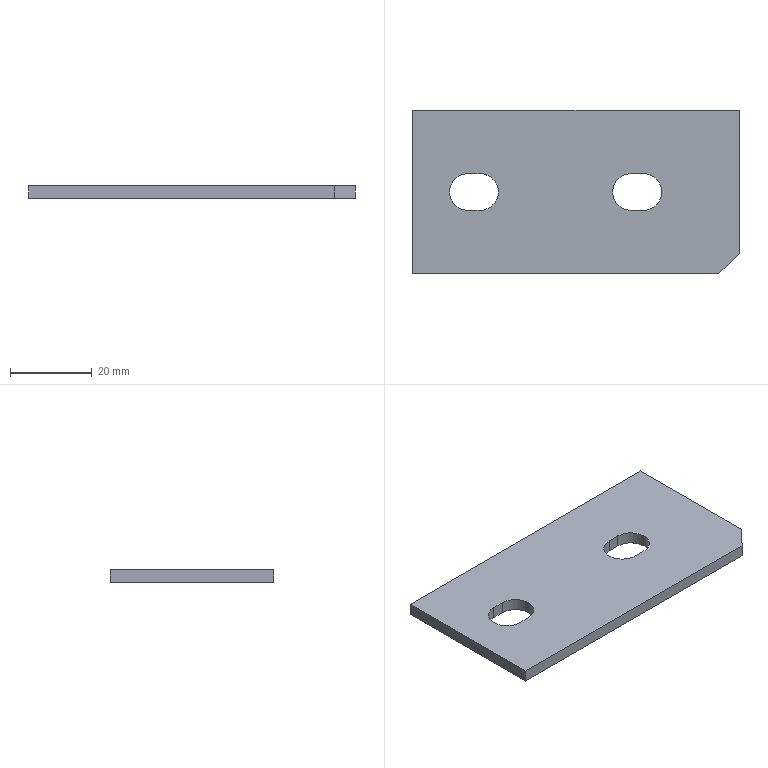Part | SolidWorks | features BaseBody 1 | 1 solid | 17 faces | box 80 x 40 x 3 mm | volume 9019 mm3 | plane 11 | cylinder 6 | commonest cylinder face diameters 9 x6
STEP:
#1=CARTESIAN_POINT('',(-26.5,-4.5,-3.));
#2=VERTEX_POINT('',#1);
#3=CARTESIAN_POINT('',(-26.5,-4.5,0.));
#4=VERTEX_POINT('',#3);
#5=CARTESIAN_POINT('',(-26.5,-4.5,-10.));
#6=DIRECTION('',(0.,0.,1.));
#7=VECTOR('',#6,1000.);
#8=LINE('',#5,#7);
#9=EDGE_CURVE('',#2,#4,#8,.T.);
#10=ORIENTED_EDGE('',*,*,#9,.T.);
#11=CARTESIAN_POINT('',(-23.5,-4.5,0.));
#12=VERTEX_POINT('',#11);
#13=CARTESIAN_POINT('',(-26.5,-4.5,0.));
#14=DIRECTION('',(1.,0.,0.));
#15=VECTOR('',#14,1000.);
#16=LINE('',#13,#15);
#17=EDGE_CURVE('',#4,#12,#16,.T.);
#18=ORIENTED_EDGE('',*,*,#17,.T.);
#19=CARTESIAN_POINT('',(-23.5,-4.5,-3.));
#20=VERTEX_POINT('',#19);
#21=CARTESIAN_POINT('',(-23.5,-4.5,-10.));
#22=DIRECTION('',(0.,0.,1.));
#23=VECTOR('',#22,1000.);
#24=LINE('',#21,#23);
#25=EDGE_CURVE('',#20,#12,#24,.T.);
#26=ORIENTED_EDGE('',*,*,#25,.F.);
#27=CARTESIAN_POINT('',(0.,-4.5,-3.));
#28=DIRECTION('',(1.,0.,0.));
#29=VECTOR('',#28,1000.);
#30=LINE('',#27,#29);
#31=EDGE_CURVE('',#2,#20,#30,.T.);
#32=ORIENTED_EDGE('',*,*,#31,.F.);
#33=EDGE_LOOP('',(#10,#18,#26,#32));
#34=FACE_OUTER_BOUND('',#33,.T.);
#35=CARTESIAN_POINT('',(-26.5,-4.5,-10.));
#36=DIRECTION('',(0.,-1.,0.));
#37=DIRECTION('',(0.,0.,-1.));
#38=AXIS2_PLACEMENT_3D('',#35,#36,#37);
#39=PLANE('',#38);
#40=ADVANCED_FACE('',(#34),#39,.F.);
#41=CARTESIAN_POINT('',(-19.,0.,-3.));
#42=VERTEX_POINT('',#41);
#43=CARTESIAN_POINT('',(-19.,0.,0.));
#44=VERTEX_POINT('',#43);
#45=CARTESIAN_POINT('',(-19.,0.,-10.));
#46=DIRECTION('',(0.,0.,1.));
#47=VECTOR('',#46,1000.);
#48=LINE('',#45,#47);
#49=EDGE_CURVE('',#42,#44,#48,.T.);
#50=ORIENTED_EDGE('',*,*,#49,.F.);
#51=CARTESIAN_POINT('',(-23.5,0.,-3.));
#52=DIRECTION('',(0.,0.,1.));
#53=DIRECTION('',(1.,0.,0.));
#54=AXIS2_PLACEMENT_3D('',#51,#52,#53);
#55=CIRCLE('',#54,4.5);
#56=EDGE_CURVE('',#20,#42,#55,.T.);
#57=ORIENTED_EDGE('',*,*,#56,.F.);
#58=ORIENTED_EDGE('',*,*,#25,.T.);
#59=CARTESIAN_POINT('',(-23.5,0.,0.));
#60=DIRECTION('',(0.,0.,1.));
#61=DIRECTION('',(1.,0.,0.));
#62=AXIS2_PLACEMENT_3D('',#59,#60,#61);
#63=CIRCLE('',#62,4.5);
#64=EDGE_CURVE('',#12,#44,#63,.T.);
#65=ORIENTED_EDGE('',*,*,#64,.T.);
#66=EDGE_LOOP('',(#50,#57,#58,#65));
#67=FACE_OUTER_BOUND('',#66,.T.);
#68=CARTESIAN_POINT('',(-23.5,0.,-10.));
#69=DIRECTION('',(0.,0.,1.));
#70=DIRECTION('',(1.,0.,0.));
#71=AXIS2_PLACEMENT_3D('',#68,#69,#70);
#72=CYLINDRICAL_SURFACE('',#71,4.5);
#73=ADVANCED_FACE('',(#67),#72,.F.);
#74=CARTESIAN_POINT('',(-23.5,4.5,-3.));
#75=VERTEX_POINT('',#74);
#76=CARTESIAN_POINT('',(-23.5,4.5,0.));
#77=VERTEX_POINT('',#76);
#78=CARTESIAN_POINT('',(-23.5,4.5,-10.));
#79=DIRECTION('',(0.,0.,1.));
#80=VECTOR('',#79,1000.);
#81=LINE('',#78,#80);
#82=EDGE_CURVE('',#75,#77,#81,.T.);
#83=ORIENTED_EDGE('',*,*,#82,.T.);
#84=CARTESIAN_POINT('',(-26.5,4.5,0.));
#85=VERTEX_POINT('',#84);
#86=CARTESIAN_POINT('',(-26.5,4.5,0.));
#87=DIRECTION('',(-1.,0.,0.));
#88=VECTOR('',#87,1000.);
#89=LINE('',#86,#88);
#90=EDGE_CURVE('',#77,#85,#89,.T.);
#91=ORIENTED_EDGE('',*,*,#90,.T.);
#92=CARTESIAN_POINT('',(-26.5,4.5,-3.));
#93=VERTEX_POINT('',#92);
#94=CARTESIAN_POINT('',(-26.5,4.5,-10.));
#95=DIRECTION('',(0.,0.,1.));
#96=VECTOR('',#95,1000.);
#97=LINE('',#94,#96);
#98=EDGE_CURVE('',#93,#85,#97,.T.);
#99=ORIENTED_EDGE('',*,*,#98,.F.);
#100=CARTESIAN_POINT('',(0.,4.5,-3.));
#101=DIRECTION('',(-1.,0.,0.));
#102=VECTOR('',#101,1000.);
#103=LINE('',#100,#102);
#104=EDGE_CURVE('',#75,#93,#103,.T.);
#105=ORIENTED_EDGE('',*,*,#104,.F.);
#106=EDGE_LOOP('',(#83,#91,#99,#105));
#107=FACE_OUTER_BOUND('',#106,.T.);
#108=CARTESIAN_POINT('',(-26.5,4.5,-10.));
#109=DIRECTION('',(0.,1.,0.));
#110=DIRECTION('',(1.,0.,0.));
#111=AXIS2_PLACEMENT_3D('',#108,#109,#110);
#112=PLANE('',#111);
#113=ADVANCED_FACE('',(#107),#112,.F.);
#114=ORIENTED_EDGE('',*,*,#98,.T.);
#115=CARTESIAN_POINT('',(-26.5,0.,0.));
#116=DIRECTION('',(0.,0.,1.));
#117=DIRECTION('',(1.,0.,0.));
#118=AXIS2_PLACEMENT_3D('',#115,#116,#117);
#119=CIRCLE('',#118,4.5);
#120=EDGE_CURVE('',#85,#4,#119,.T.);
#121=ORIENTED_EDGE('',*,*,#120,.T.);
#122=ORIENTED_EDGE('',*,*,#9,.F.);
#123=CARTESIAN_POINT('',(-26.5,0.,-3.));
#124=DIRECTION('',(0.,0.,1.));
#125=DIRECTION('',(1.,0.,0.));
#126=AXIS2_PLACEMENT_3D('',#123,#124,#125);
#127=CIRCLE('',#126,4.5);
#128=EDGE_CURVE('',#93,#2,#127,.T.);
#129=ORIENTED_EDGE('',*,*,#128,.F.);
#130=EDGE_LOOP('',(#114,#121,#122,#129));
#131=FACE_OUTER_BOUND('',#130,.T.);
#132=CARTESIAN_POINT('',(-26.5,0.,-10.));
#133=DIRECTION('',(0.,0.,1.));
#134=DIRECTION('',(1.,0.,0.));
#135=AXIS2_PLACEMENT_3D('',#132,#133,#134);
#136=CYLINDRICAL_SURFACE('',#135,4.5);
#137=ADVANCED_FACE('',(#131),#136,.F.);
#138=CARTESIAN_POINT('',(16.5,4.5,-3.));
#139=VERTEX_POINT('',#138);
#140=CARTESIAN_POINT('',(16.5,4.5,0.));
#141=VERTEX_POINT('',#140);
#142=CARTESIAN_POINT('',(16.5,4.5,-10.));
#143=DIRECTION('',(0.,0.,1.));
#144=VECTOR('',#143,1000.);
#145=LINE('',#142,#144);
#146=EDGE_CURVE('',#139,#141,#145,.T.);
#147=ORIENTED_EDGE('',*,*,#146,.T.);
#148=CARTESIAN_POINT('',(13.5,4.5,0.));
#149=VERTEX_POINT('',#148);
#150=CARTESIAN_POINT('',(16.5,4.5,0.));
#151=DIRECTION('',(-1.,0.,0.));
#152=VECTOR('',#151,1000.);
#153=LINE('',#150,#152);
#154=EDGE_CURVE('',#141,#149,#153,.T.);
#155=ORIENTED_EDGE('',*,*,#154,.T.);
#156=CARTESIAN_POINT('',(13.5,4.5,-3.));
#157=VERTEX_POINT('',#156);
#158=CARTESIAN_POINT('',(13.5,4.5,-10.));
#159=DIRECTION('',(0.,0.,1.));
#160=VECTOR('',#159,1000.);
#161=LINE('',#158,#160);
#162=EDGE_CURVE('',#157,#149,#161,.T.);
#163=ORIENTED_EDGE('',*,*,#162,.F.);
#164=CARTESIAN_POINT('',(0.,4.5,-3.));
#165=DIRECTION('',(-1.,0.,0.));
#166=VECTOR('',#165,1000.);
#167=LINE('',#164,#166);
#168=EDGE_CURVE('',#139,#157,#167,.T.);
#169=ORIENTED_EDGE('',*,*,#168,.F.);
#170=EDGE_LOOP('',(#147,#155,#163,#169));
#171=FACE_OUTER_BOUND('',#170,.T.);
#172=CARTESIAN_POINT('',(16.5,4.5,-10.));
#173=DIRECTION('',(0.,1.,0.));
#174=DIRECTION('',(1.,0.,0.));
#175=AXIS2_PLACEMENT_3D('',#172,#173,#174);
#176=PLANE('',#175);
#177=ADVANCED_FACE('',(#171),#176,.F.);
#178=ORIENTED_EDGE('',*,*,#162,.T.);
#179=CARTESIAN_POINT('',(13.5,-4.5,0.));
#180=VERTEX_POINT('',#179);
#181=CARTESIAN_POINT('',(13.5,0.,0.));
#182=DIRECTION('',(0.,0.,1.));
#183=DIRECTION('',(-1.,0.,0.));
#184=AXIS2_PLACEMENT_3D('',#181,#182,#183);
#185=CIRCLE('',#184,4.5);
#186=EDGE_CURVE('',#149,#180,#185,.T.);
#187=ORIENTED_EDGE('',*,*,#186,.T.);
#188=CARTESIAN_POINT('',(13.5,-4.5,-3.));
#189=VERTEX_POINT('',#188);
#190=CARTESIAN_POINT('',(13.5,-4.5,-10.));
#191=DIRECTION('',(0.,0.,1.));
#192=VECTOR('',#191,1000.);
#193=LINE('',#190,#192);
#194=EDGE_CURVE('',#189,#180,#193,.T.);
#195=ORIENTED_EDGE('',*,*,#194,.F.);
#196=CARTESIAN_POINT('',(13.5,0.,-3.));
#197=DIRECTION('',(0.,0.,1.));
#198=DIRECTION('',(1.,0.,0.));
#199=AXIS2_PLACEMENT_3D('',#196,#197,#198);
#200=CIRCLE('',#199,4.5);
#201=EDGE_CURVE('',#157,#189,#200,.T.);
#202=ORIENTED_EDGE('',*,*,#201,.F.);
#203=EDGE_LOOP('',(#178,#187,#195,#202));
#204=FACE_OUTER_BOUND('',#203,.T.);
#205=CARTESIAN_POINT('',(13.5,0.,-10.));
#206=DIRECTION('',(0.,0.,1.));
#207=DIRECTION('',(1.,0.,0.));
#208=AXIS2_PLACEMENT_3D('',#205,#206,#207);
#209=CYLINDRICAL_SURFACE('',#208,4.5);
#210=ADVANCED_FACE('',(#204),#209,.F.);
#211=ORIENTED_EDGE('',*,*,#194,.T.);
#212=CARTESIAN_POINT('',(16.5,-4.5,0.));
#213=VERTEX_POINT('',#212);
#214=CARTESIAN_POINT('',(16.5,-4.5,0.));
#215=DIRECTION('',(1.,0.,0.));
#216=VECTOR('',#215,1000.);
#217=LINE('',#214,#216);
#218=EDGE_CURVE('',#180,#213,#217,.T.);
#219=ORIENTED_EDGE('',*,*,#218,.T.);
#220=CARTESIAN_POINT('',(16.5,-4.5,-3.));
#221=VERTEX_POINT('',#220);
#222=CARTESIAN_POINT('',(16.5,-4.5,-10.));
#223=DIRECTION('',(0.,0.,1.));
#224=VECTOR('',#223,1000.);
#225=LINE('',#222,#224);
#226=EDGE_CURVE('',#221,#213,#225,.T.);
#227=ORIENTED_EDGE('',*,*,#226,.F.);
#228=CARTESIAN_POINT('',(0.,-4.5,-3.));
#229=DIRECTION('',(1.,0.,0.));
#230=VECTOR('',#229,1000.);
#231=LINE('',#228,#230);
#232=EDGE_CURVE('',#189,#221,#231,.T.);
#233=ORIENTED_EDGE('',*,*,#232,.F.);
#234=EDGE_LOOP('',(#211,#219,#227,#233));
#235=FACE_OUTER_BOUND('',#234,.T.);
#236=CARTESIAN_POINT('',(16.5,-4.5,-10.));
#237=DIRECTION('',(0.,-1.,0.));
#238=DIRECTION('',(0.,0.,-1.));
#239=AXIS2_PLACEMENT_3D('',#236,#237,#238);
#240=PLANE('',#239);
#241=ADVANCED_FACE('',(#235),#240,.F.);
#242=CARTESIAN_POINT('',(21.,0.,-3.));
#243=VERTEX_POINT('',#242);
#244=CARTESIAN_POINT('',(21.,0.,0.));
#245=VERTEX_POINT('',#244);
#246=CARTESIAN_POINT('',(21.,0.,-10.));
#247=DIRECTION('',(0.,0.,1.));
#248=VECTOR('',#247,1000.);
#249=LINE('',#246,#248);
#250=EDGE_CURVE('',#243,#245,#249,.T.);
#251=ORIENTED_EDGE('',*,*,#250,.F.);
#252=CARTESIAN_POINT('',(16.5,0.,-3.));
#253=DIRECTION('',(0.,0.,1.));
#254=DIRECTION('',(1.,0.,0.));
#255=AXIS2_PLACEMENT_3D('',#252,#253,#254);
#256=CIRCLE('',#255,4.5);
#257=EDGE_CURVE('',#221,#243,#256,.T.);
#258=ORIENTED_EDGE('',*,*,#257,.F.);
#259=ORIENTED_EDGE('',*,*,#226,.T.);
#260=CARTESIAN_POINT('',(16.5,0.,0.));
#261=DIRECTION('',(0.,0.,1.));
#262=DIRECTION('',(-1.,0.,0.));
#263=AXIS2_PLACEMENT_3D('',#260,#261,#262);
#264=CIRCLE('',#263,4.5);
#265=EDGE_CURVE('',#213,#245,#264,.T.);
#266=ORIENTED_EDGE('',*,*,#265,.T.);
#267=EDGE_LOOP('',(#251,#258,#259,#266));
#268=FACE_OUTER_BOUND('',#267,.T.);
#269=CARTESIAN_POINT('',(16.5,0.,-10.));
#270=DIRECTION('',(0.,0.,1.));
#271=DIRECTION('',(1.,0.,0.));
#272=AXIS2_PLACEMENT_3D('',#269,#270,#271);
#273=CYLINDRICAL_SURFACE('',#272,4.5);
#274=ADVANCED_FACE('',(#268),#273,.F.);
#275=CARTESIAN_POINT('',(40.,-15.,-3.));
#276=VERTEX_POINT('',#275);
#277=CARTESIAN_POINT('',(35.,-20.,-3.));
#278=VERTEX_POINT('',#277);
#279=CARTESIAN_POINT('',(35.,-20.,-3.));
#280=DIRECTION('',(-0.7071,-0.7071,0.));
#281=VECTOR('',#280,1000.);
#282=LINE('',#279,#281);
#283=EDGE_CURVE('',#276,#278,#282,.T.);
#284=ORIENTED_EDGE('',*,*,#283,.F.);
#285=CARTESIAN_POINT('',(40.,-15.,0.));
#286=VERTEX_POINT('',#285);
#287=CARTESIAN_POINT('',(40.,-15.,-3.));
#288=DIRECTION('',(0.,0.,-1.));
#289=VECTOR('',#288,1000.);
#290=LINE('',#287,#289);
#291=EDGE_CURVE('',#286,#276,#290,.T.);
#292=ORIENTED_EDGE('',*,*,#291,.F.);
#293=CARTESIAN_POINT('',(35.,-20.,0.));
#294=VERTEX_POINT('',#293);
#295=CARTESIAN_POINT('',(27.5,-27.5,0.));
#296=DIRECTION('',(0.7071,0.7071,0.));
#297=VECTOR('',#296,1000.);
#298=LINE('',#295,#297);
#299=EDGE_CURVE('',#294,#286,#298,.T.);
#300=ORIENTED_EDGE('',*,*,#299,.F.);
#301=CARTESIAN_POINT('',(35.,-20.,-3.));
#302=DIRECTION('',(0.,0.,1.));
#303=VECTOR('',#302,1000.);
#304=LINE('',#301,#303);
#305=EDGE_CURVE('',#278,#294,#304,.T.);
#306=ORIENTED_EDGE('',*,*,#305,.F.);
#307=EDGE_LOOP('',(#284,#292,#300,#306));
#308=FACE_OUTER_BOUND('',#307,.T.);
#309=CARTESIAN_POINT('',(35.,-20.,-3.));
#310=DIRECTION('',(-0.7071,0.7071,0.));
#311=DIRECTION('',(0.,0.,1.));
#312=AXIS2_PLACEMENT_3D('',#309,#310,#311);
#313=PLANE('',#312);
#314=ADVANCED_FACE('',(#308),#313,.F.);
#315=ORIENTED_EDGE('',*,*,#265,.F.);
#316=ORIENTED_EDGE('',*,*,#218,.F.);
#317=ORIENTED_EDGE('',*,*,#186,.F.);
#318=ORIENTED_EDGE('',*,*,#154,.F.);
#319=CARTESIAN_POINT('',(16.5,0.,0.));
#320=DIRECTION('',(0.,0.,1.));
#321=DIRECTION('',(-1.,0.,0.));
#322=AXIS2_PLACEMENT_3D('',#319,#320,#321);
#323=CIRCLE('',#322,4.5);
#324=EDGE_CURVE('',#245,#141,#323,.T.);
#325=ORIENTED_EDGE('',*,*,#324,.F.);
#326=EDGE_LOOP('',(#315,#316,#317,#318,#325));
#327=FACE_BOUND('',#326,.T.);
#328=ORIENTED_EDGE('',*,*,#120,.F.);
#329=ORIENTED_EDGE('',*,*,#90,.F.);
#330=CARTESIAN_POINT('',(-23.5,0.,0.));
#331=DIRECTION('',(0.,0.,1.));
#332=DIRECTION('',(1.,0.,0.));
#333=AXIS2_PLACEMENT_3D('',#330,#331,#332);
#334=CIRCLE('',#333,4.5);
#335=EDGE_CURVE('',#44,#77,#334,.T.);
#336=ORIENTED_EDGE('',*,*,#335,.F.);
#337=ORIENTED_EDGE('',*,*,#64,.F.);
#338=ORIENTED_EDGE('',*,*,#17,.F.);
#339=EDGE_LOOP('',(#328,#329,#336,#337,#338));
#340=FACE_BOUND('',#339,.T.);
#341=CARTESIAN_POINT('',(-40.,-20.,0.));
#342=VERTEX_POINT('',#341);
#343=CARTESIAN_POINT('',(-40.,-20.,0.));
#344=DIRECTION('',(1.,0.,0.));
#345=VECTOR('',#344,1000.);
#346=LINE('',#343,#345);
#347=EDGE_CURVE('',#342,#294,#346,.T.);
#348=ORIENTED_EDGE('',*,*,#347,.T.);
#349=ORIENTED_EDGE('',*,*,#299,.T.);
#350=CARTESIAN_POINT('',(40.,20.,0.));
#351=VERTEX_POINT('',#350);
#352=CARTESIAN_POINT('',(40.,20.,0.));
#353=DIRECTION('',(0.,1.,0.));
#354=VECTOR('',#353,1000.);
#355=LINE('',#352,#354);
#356=EDGE_CURVE('',#286,#351,#355,.T.);
#357=ORIENTED_EDGE('',*,*,#356,.T.);
#358=CARTESIAN_POINT('',(-40.,20.,0.));
#359=VERTEX_POINT('',#358);
#360=CARTESIAN_POINT('',(-40.,20.,0.));
#361=DIRECTION('',(-1.,0.,0.));
#362=VECTOR('',#361,1000.);
#363=LINE('',#360,#362);
#364=EDGE_CURVE('',#351,#359,#363,.T.);
#365=ORIENTED_EDGE('',*,*,#364,.T.);
#366=CARTESIAN_POINT('',(-40.,20.,0.));
#367=DIRECTION('',(0.,-1.,0.));
#368=VECTOR('',#367,1000.);
#369=LINE('',#366,#368);
#370=EDGE_CURVE('',#359,#342,#369,.T.);
#371=ORIENTED_EDGE('',*,*,#370,.T.);
#372=EDGE_LOOP('',(#348,#349,#357,#365,#371));
#373=FACE_OUTER_BOUND('',#372,.T.);
#374=CARTESIAN_POINT('',(0.,0.,0.));
#375=DIRECTION('',(0.,0.,1.));
#376=DIRECTION('',(1.,0.,0.));
#377=AXIS2_PLACEMENT_3D('',#374,#375,#376);
#378=PLANE('',#377);
#379=ADVANCED_FACE('',(#327,#340,#373),#378,.T.);
#380=ORIENTED_EDGE('',*,*,#232,.T.);
#381=ORIENTED_EDGE('',*,*,#257,.T.);
#382=CARTESIAN_POINT('',(16.5,0.,-3.));
#383=DIRECTION('',(0.,0.,1.));
#384=DIRECTION('',(1.,0.,0.));
#385=AXIS2_PLACEMENT_3D('',#382,#383,#384);
#386=CIRCLE('',#385,4.5);
#387=EDGE_CURVE('',#243,#139,#386,.T.);
#388=ORIENTED_EDGE('',*,*,#387,.T.);
#389=ORIENTED_EDGE('',*,*,#168,.T.);
#390=ORIENTED_EDGE('',*,*,#201,.T.);
#391=EDGE_LOOP('',(#380,#381,#388,#389,#390));
#392=FACE_BOUND('',#391,.T.);
#393=ORIENTED_EDGE('',*,*,#104,.T.);
#394=ORIENTED_EDGE('',*,*,#128,.T.);
#395=ORIENTED_EDGE('',*,*,#31,.T.);
#396=ORIENTED_EDGE('',*,*,#56,.T.);
#397=CARTESIAN_POINT('',(-23.5,0.,-3.));
#398=DIRECTION('',(0.,0.,1.));
#399=DIRECTION('',(1.,0.,0.));
#400=AXIS2_PLACEMENT_3D('',#397,#398,#399);
#401=CIRCLE('',#400,4.5);
#402=EDGE_CURVE('',#42,#75,#401,.T.);
#403=ORIENTED_EDGE('',*,*,#402,.T.);
#404=EDGE_LOOP('',(#393,#394,#395,#396,#403));
#405=FACE_BOUND('',#404,.T.);
#406=CARTESIAN_POINT('',(40.,20.,-3.));
#407=VERTEX_POINT('',#406);
#408=CARTESIAN_POINT('',(40.,20.,-3.));
#409=DIRECTION('',(0.,1.,0.));
#410=VECTOR('',#409,1000.);
#411=LINE('',#408,#410);
#412=EDGE_CURVE('',#276,#407,#411,.T.);
#413=ORIENTED_EDGE('',*,*,#412,.F.);
#414=ORIENTED_EDGE('',*,*,#283,.T.);
#415=CARTESIAN_POINT('',(-40.,-20.,-3.));
#416=VERTEX_POINT('',#415);
#417=CARTESIAN_POINT('',(-40.,-20.,-3.));
#418=DIRECTION('',(1.,0.,0.));
#419=VECTOR('',#418,1000.);
#420=LINE('',#417,#419);
#421=EDGE_CURVE('',#416,#278,#420,.T.);
#422=ORIENTED_EDGE('',*,*,#421,.F.);
#423=CARTESIAN_POINT('',(-40.,20.,-3.));
#424=VERTEX_POINT('',#423);
#425=CARTESIAN_POINT('',(-40.,20.,-3.));
#426=DIRECTION('',(0.,-1.,0.));
#427=VECTOR('',#426,1000.);
#428=LINE('',#425,#427);
#429=EDGE_CURVE('',#424,#416,#428,.T.);
#430=ORIENTED_EDGE('',*,*,#429,.F.);
#431=CARTESIAN_POINT('',(-40.,20.,-3.));
#432=DIRECTION('',(-1.,0.,0.));
#433=VECTOR('',#432,1000.);
#434=LINE('',#431,#433);
#435=EDGE_CURVE('',#407,#424,#434,.T.);
#436=ORIENTED_EDGE('',*,*,#435,.F.);
#437=EDGE_LOOP('',(#413,#414,#422,#430,#436));
#438=FACE_OUTER_BOUND('',#437,.T.);
#439=CARTESIAN_POINT('',(0.,0.,-3.));
#440=DIRECTION('',(0.,0.,1.));
#441=DIRECTION('',(1.,0.,0.));
#442=AXIS2_PLACEMENT_3D('',#439,#440,#441);
#443=PLANE('',#442);
#444=ADVANCED_FACE('',(#392,#405,#438),#443,.F.);
#445=ORIENTED_EDGE('',*,*,#364,.F.);
#446=CARTESIAN_POINT('',(40.,20.,-3.));
#447=DIRECTION('',(0.,0.,1.));
#448=VECTOR('',#447,1000.);
#449=LINE('',#446,#448);
#450=EDGE_CURVE('',#407,#351,#449,.T.);
#451=ORIENTED_EDGE('',*,*,#450,.F.);
#452=ORIENTED_EDGE('',*,*,#435,.T.);
#453=CARTESIAN_POINT('',(-40.,20.,-3.));
#454=DIRECTION('',(0.,0.,1.));
#455=VECTOR('',#454,1000.);
#456=LINE('',#453,#455);
#457=EDGE_CURVE('',#424,#359,#456,.T.);
#458=ORIENTED_EDGE('',*,*,#457,.T.);
#459=EDGE_LOOP('',(#445,#451,#452,#458));
#460=FACE_OUTER_BOUND('',#459,.T.);
#461=CARTESIAN_POINT('',(-40.,20.,-3.));
#462=DIRECTION('',(0.,1.,0.));
#463=DIRECTION('',(1.,0.,0.));
#464=AXIS2_PLACEMENT_3D('',#461,#462,#463);
#465=PLANE('',#464);
#466=ADVANCED_FACE('',(#460),#465,.T.);
#467=ORIENTED_EDGE('',*,*,#370,.F.);
#468=ORIENTED_EDGE('',*,*,#457,.F.);
#469=ORIENTED_EDGE('',*,*,#429,.T.);
#470=CARTESIAN_POINT('',(-40.,-20.,-3.));
#471=DIRECTION('',(0.,0.,1.));
#472=VECTOR('',#471,1000.);
#473=LINE('',#470,#472);
#474=EDGE_CURVE('',#416,#342,#473,.T.);
#475=ORIENTED_EDGE('',*,*,#474,.T.);
#476=EDGE_LOOP('',(#467,#468,#469,#475));
#477=FACE_OUTER_BOUND('',#476,.T.);
#478=CARTESIAN_POINT('',(-40.,20.,-3.));
#479=DIRECTION('',(-1.,0.,0.));
#480=DIRECTION('',(0.,1.,0.));
#481=AXIS2_PLACEMENT_3D('',#478,#479,#480);
#482=PLANE('',#481);
#483=ADVANCED_FACE('',(#477),#482,.T.);
#484=ORIENTED_EDGE('',*,*,#421,.T.);
#485=ORIENTED_EDGE('',*,*,#305,.T.);
#486=ORIENTED_EDGE('',*,*,#347,.F.);
#487=ORIENTED_EDGE('',*,*,#474,.F.);
#488=EDGE_LOOP('',(#484,#485,#486,#487));
#489=FACE_OUTER_BOUND('',#488,.T.);
#490=CARTESIAN_POINT('',(-40.,-20.,-3.));
#491=DIRECTION('',(0.,-1.,0.));
#492=DIRECTION('',(0.,0.,-1.));
#493=AXIS2_PLACEMENT_3D('',#490,#491,#492);
#494=PLANE('',#493);
#495=ADVANCED_FACE('',(#489),#494,.T.);
#496=ORIENTED_EDGE('',*,*,#356,.F.);
#497=ORIENTED_EDGE('',*,*,#291,.T.);
#498=ORIENTED_EDGE('',*,*,#412,.T.);
#499=ORIENTED_EDGE('',*,*,#450,.T.);
#500=EDGE_LOOP('',(#496,#497,#498,#499));
#501=FACE_OUTER_BOUND('',#500,.T.);
#502=CARTESIAN_POINT('',(40.,20.,-3.));
#503=DIRECTION('',(1.,0.,0.));
#504=DIRECTION('',(0.,-1.,0.));
#505=AXIS2_PLACEMENT_3D('',#502,#503,#504);
#506=PLANE('',#505);
#507=ADVANCED_FACE('',(#501),#506,.T.);
#508=ORIENTED_EDGE('',*,*,#387,.F.);
#509=ORIENTED_EDGE('',*,*,#250,.T.);
#510=ORIENTED_EDGE('',*,*,#324,.T.);
#511=ORIENTED_EDGE('',*,*,#146,.F.);
#512=EDGE_LOOP('',(#508,#509,#510,#511));
#513=FACE_OUTER_BOUND('',#512,.T.);
#514=CARTESIAN_POINT('',(16.5,0.,-10.));
#515=DIRECTION('',(0.,0.,1.));
#516=DIRECTION('',(1.,0.,0.));
#517=AXIS2_PLACEMENT_3D('',#514,#515,#516);
#518=CYLINDRICAL_SURFACE('',#517,4.5);
#519=ADVANCED_FACE('',(#513),#518,.F.);
#520=ORIENTED_EDGE('',*,*,#402,.F.);
#521=ORIENTED_EDGE('',*,*,#49,.T.);
#522=ORIENTED_EDGE('',*,*,#335,.T.);
#523=ORIENTED_EDGE('',*,*,#82,.F.);
#524=EDGE_LOOP('',(#520,#521,#522,#523));
#525=FACE_OUTER_BOUND('',#524,.T.);
#526=CARTESIAN_POINT('',(-23.5,0.,-10.));
#527=DIRECTION('',(0.,0.,1.));
#528=DIRECTION('',(1.,0.,0.));
#529=AXIS2_PLACEMENT_3D('',#526,#527,#528);
#530=CYLINDRICAL_SURFACE('',#529,4.5);
#531=ADVANCED_FACE('',(#525),#530,.F.);
#532=CLOSED_SHELL('',(#40,#73,#113,#137,#177,#210,#241,#274,#314,#379,#444,#466,#483,#495,#507,#519,#531));
#533=MANIFOLD_SOLID_BREP('',#532);
#534=CARTESIAN_POINT('',(0.,0.,0.));
#535=DIRECTION('',(0.,0.,1.));
#536=DIRECTION('',(1.,0.,0.));
#537=AXIS2_PLACEMENT_3D('',#534,#535,#536);
#538=(LENGTH_UNIT()NAMED_UNIT(*)SI_UNIT(.MILLI.,.METRE.));
#539=UNCERTAINTY_MEASURE_WITH_UNIT(LENGTH_MEASURE(0.00001),#538,'','');
#540=(NAMED_UNIT(*)PLANE_ANGLE_UNIT()SI_UNIT($,.RADIAN.));
#541=(NAMED_UNIT(*)SI_UNIT($,.STERADIAN.)SOLID_ANGLE_UNIT());
#542=(GEOMETRIC_REPRESENTATION_CONTEXT(3)GLOBAL_UNCERTAINTY_ASSIGNED_CONTEXT((#539))GLOBAL_UNIT_ASSIGNED_CONTEXT((#538,#540,#541))REPRESENTATION_CONTEXT('',''));
#543=ADVANCED_BREP_SHAPE_REPRESENTATION('',(#533,#537),#542);